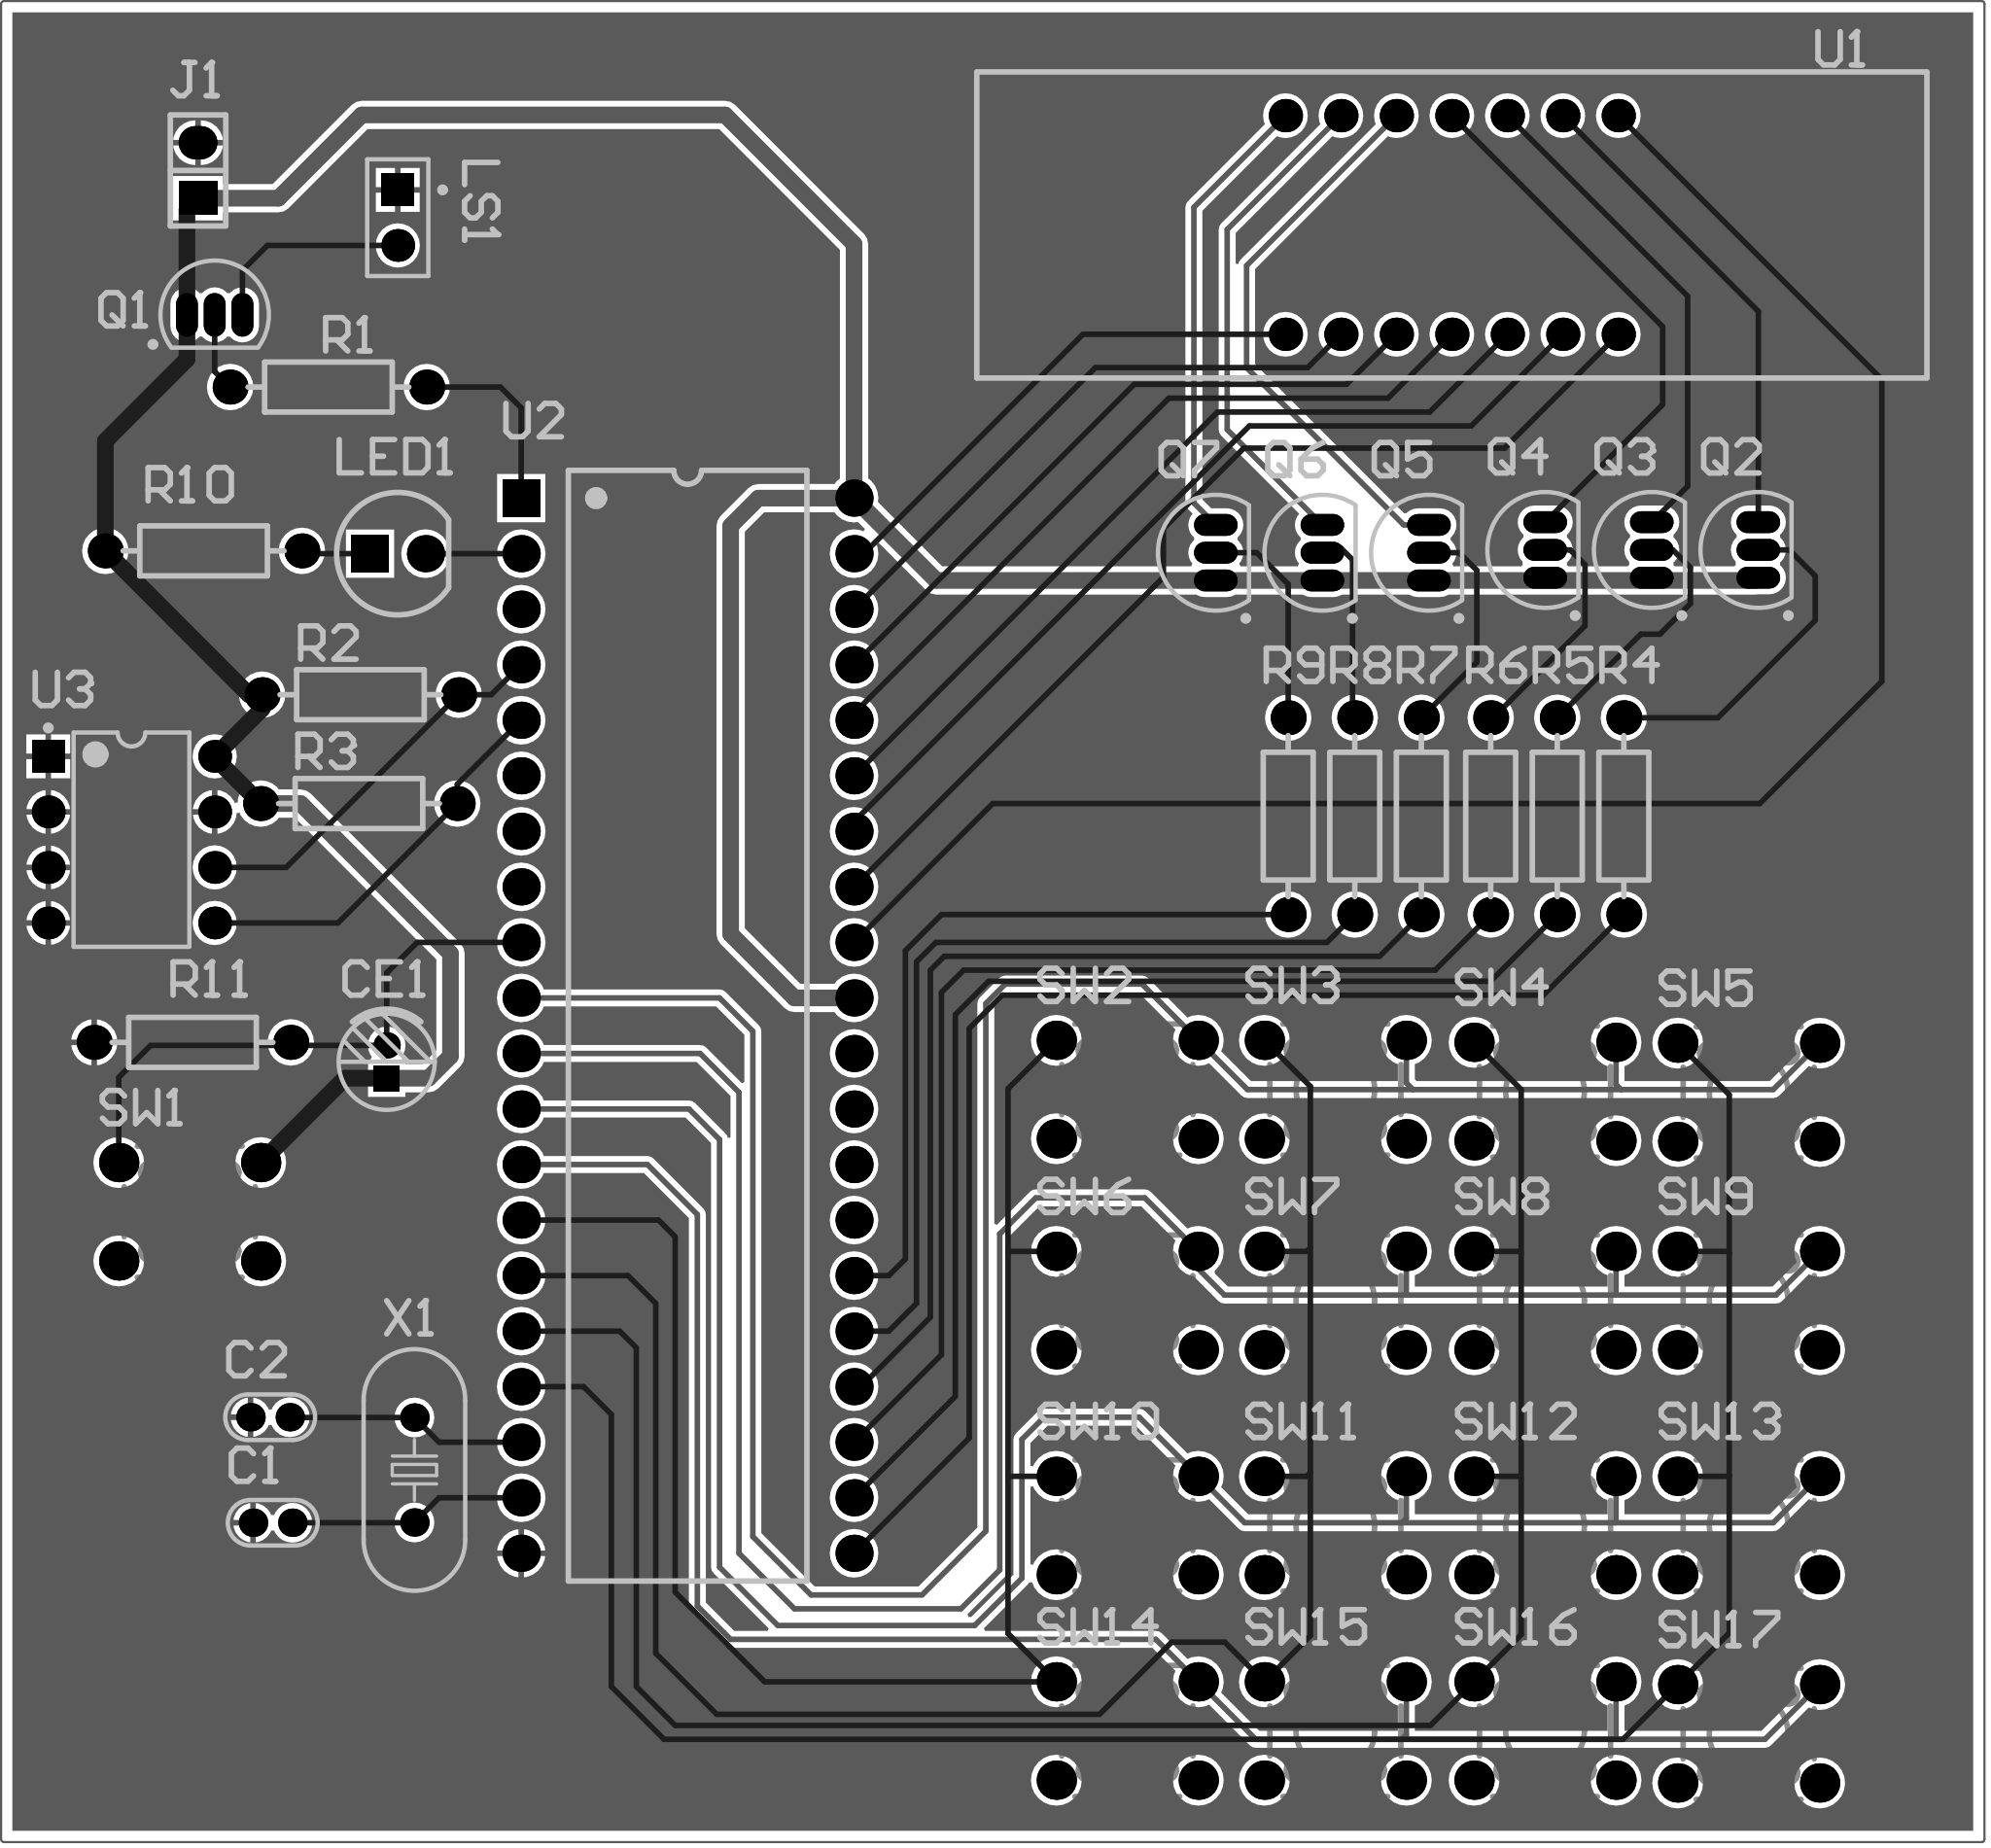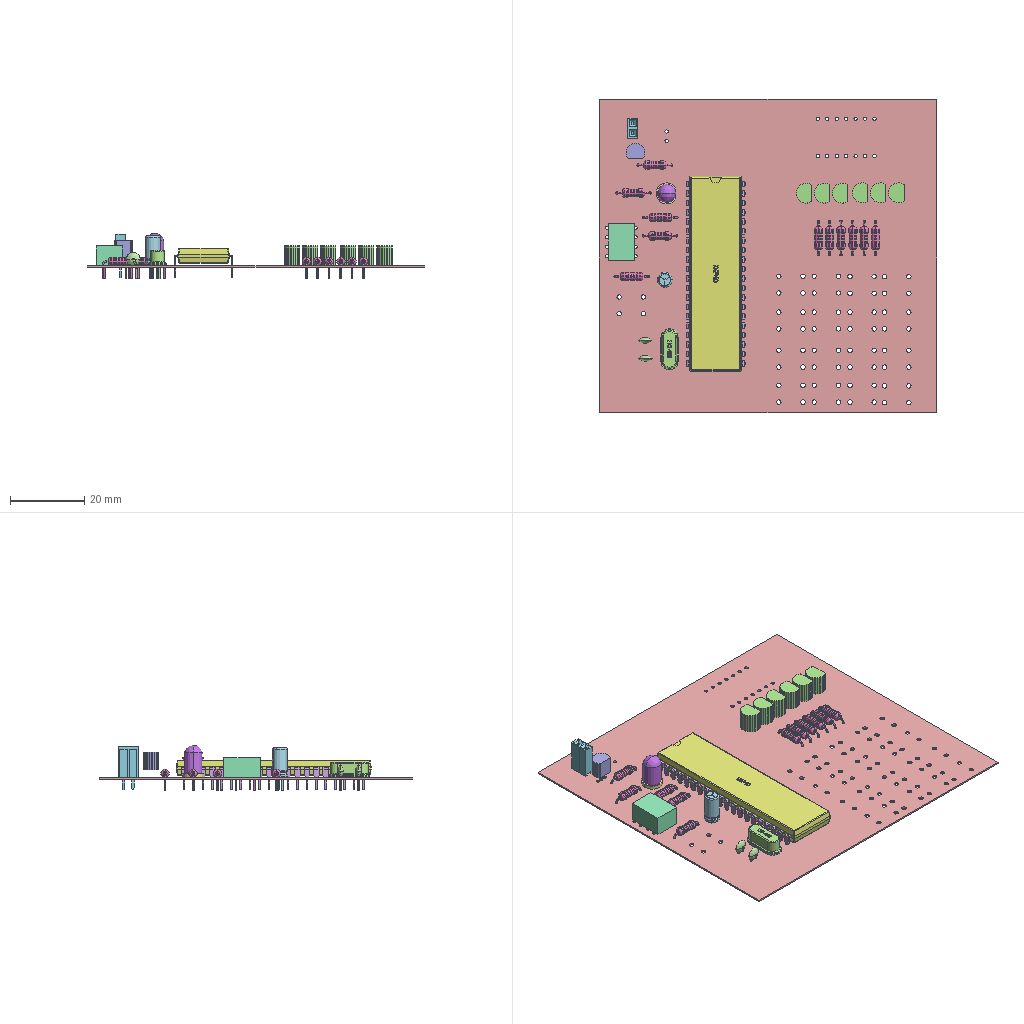Circuit board layout | Altium Designer | box 90.8 x 84.2 x 12.3 mm
Layer stack:
# Altium Designer layer stack of  (unit mm; dielectric type: 0 none, 1 core, 2 prepreg, 3 surface material)
index,name,kind,layer,copper_thickness_mm,dielectric_type,dielectric_thickness_mm,dielectric_material,dielectric_constant
0,Top Paste,other,,,,,,
1,Top Overlay,other,,,,,,
2,Top Solder,dielectric,,,3,0.0102,Solder Resist,3.5
3,Top Layer,copper,Top Layer,0.0356,,,,
4,Dielectric 1,dielectric,,,0,0.32,FR-4,4.8
5,Bottom Layer,copper,Bottom Layer,0.0356,,,,
6,Bottom Solder,dielectric,,,3,0.0102,Solder Resist,3.5
7,Bottom Overlay,other,,,,,,
8,Bottom Paste,other,,,,,,
# drill layer pairs: low layer,high layer
drill_pair,Top Layer,Bottom Layer
Part placement:
Designator,Comment,Layer,Footprint,Center-X(mm),Center-Y(mm),Rotation
C1,30PF,TopLayer,CC_1.8*3.6,35.422,57.531,0
C2,30PF,TopLayer,CC_1.8*3.6,35.306,62.357,0
CE1,47UF,TopLayer,CAP_1.5*4*8,40.64,78.613,90
LED1,Red,TopLayer,LED_5MM-B,41.148,101.854,0
LS1,Bell,TopLayer,PIN2,41.148,117.221,270
Q1,PNP,TopLayer,TO-92A,32.766,112.776,270
Q2,NPN,TopLayer,TO-226-AA,103.44,102.025,360
Q3,NPN,TopLayer,TO-226-AA,98.561,102.025,360
Q4,NPN,TopLayer,TO-226-AA,93.682,102.025,360
Q5,NPN,TopLayer,TO-226-AA,88.359,101.898,360
Q6,NPN,TopLayer,TO-226-AA,83.48,101.898,360
Q7,NPN,TopLayer,TO-226-AA,78.601,101.898,360
R1,470,TopLayer,RS_1/4W,37.973,109.474,180
R2,10K,TopLayer,RS_1/4W,39.438,95.403,180
R3,10K,TopLayer,RS_1/4W,39.37,90.424,180
R4,1K,TopLayer,RS_1/4W,97.282,89.848,90
R5,1K,TopLayer,RS_1/4W,94.234,89.848,90
R6,1K,TopLayer,RS_1/4W,91.186,89.848,90
R7,1K,TopLayer,RS_1/4W,88.011,89.848,90
R8,1K,TopLayer,RS_1/4W,84.963,89.848,90
R9,1K,TopLayer,RS_1/4W,81.915,89.848,90
R10,100,TopLayer,RS_1/4W,32.258,101.981,180
R11,1K,TopLayer,RS_1/4W,31.75,79.502,360
SW1,3x6x5,TopLayer,四脚轻触开关,31.623,71.755,0
SW2,3x6x5,TopLayer,四脚轻触开关,74.549,77.343,360
SW3,3x6x5,TopLayer,四脚轻触开关,84.074,77.343,360
SW4,3x6x5,TopLayer,四脚轻触开关,93.674,77.252,360
SW5,3x6x5,TopLayer,四脚轻触开关,102.997,77.216,360
SW6,3x6x5,TopLayer,四脚轻触开关,74.549,67.691,360
SW7,3x6x5,TopLayer,四脚轻触开关,84.074,67.691,360
SW8,3x6x5,TopLayer,四脚轻触开关,93.674,67.691,360
SW9,3x6x5,TopLayer,四脚轻触开关,102.997,67.691,360
SW10,3x6x5,TopLayer,四脚轻触开关,74.549,57.404,360
SW11,3x6x5,TopLayer,四脚轻触开关,84.074,57.404,360
SW12,3x6x5,TopLayer,四脚轻触开关,93.674,57.404,360
SW13,3x6x5,TopLayer,四脚轻触开关,102.997,57.404,360
SW14,3x6x5,TopLayer,四脚轻触开关,74.549,48.006,360
SW15,3x6x5,TopLayer,四脚轻触开关,84.074,48.006,360
SW16,3x6x5,TopLayer,四脚轻触开关,93.674,48.006,360
SW17,3x6x5,TopLayer,四脚轻触开关,102.997,47.879,360
U1,6-digit display_1,TopLayer,6位数码管,89.408,116.887,360
U2,ATC89C52,TopLayer,DIP40,54.419,80.264,0
U3,24C02C,TopLayer,PDIP300-P8,28.956,88.773,0
X1,12MHz,TopLayer,OSC_HC-49S,41.91,59.944,270
J1,Female HDR1X2,TopLayer,Fe-HDR1X2/2.54-S,32.004,119.38,90
Pad and via stacks:
# Altium Designer via and pad stacks of  (unit mm). Each distinct definition once, with the count of objects using it.
# via: kind,start_layer,end_layer,hole_mm,diameter_mm,mode(0 simple;1 top-mid-bottom;2 full stack),diameter_per_layer,count,example_net
# pad: kind,layer,hole_mm,hole_type(0 round;1 square;2 slot),plating,top_size,top_shape(1 round;2 rect;3 octagon;9 rounded rect),mid_size,bottom_size,mode,footprint,size_per_layer,count,example
pad,Multi-Layer,1.2,0,plated,1.8x1.8,1,1.8x1.8,1.8x1.8,0,\u00CB\u00C4\u00BD\u00C5\u00C7\u00E1\u00B4\u00A5\u00BF\u00AA\u00B9\u00D8,,68,SW14.1
pad,Multi-Layer,0.6,0,plated,1.6x1.6,1,1.6x1.6,1.6x1.6,0,RS 1/4W,,22,R11.1
pad,Multi-Layer,0.6,0,plated,1.2x1.2,2,1.2x1.2,1.2x1.2,0,CAP 1.5*4*8,,1,CE1.1
pad,Multi-Layer,0.6,0,plated,1.2x1.2,1,1.2x1.2,1.2x1.2,0,CAP 1.5*4*8,,1,CE1.2
pad,Multi-Layer,0.5,0,plated,1.3x1.3,1,1.3x1.3,1.3x1.3,0,CC 1.8*3.6,,4,C2.1
pad,Multi-Layer,0.6,0,plated,1.3x1.3,1,1.3x1.3,1.3x1.3,0,OSC HC-49S,,2,X1.1
pad,Multi-Layer,0.9,0,plated,1.7x1.7,1,1.7x1.7,1.7x1.7,0,LED 5MM-B,,1,LED1.2
pad,Multi-Layer,0.9,0,plated,1.7x1.7,2,1.7x1.7,1.7x1.7,0,LED 5MM-B,,1,LED1.1
pad,Multi-Layer,0.9,0,plated,1.5x1.5,2,1.5x1.5,1.5x1.5,0,PDIP300-P8,,1,U3.1
pad,Multi-Layer,0.9,0,plated,1.5x1.5,1,1.5x1.5,1.5x1.5,0,PDIP300-P8,,7,U3.2
pad,Multi-Layer,0.9,0,plated,2x1,1,2x1,2x1,0,TO-226-AA,,18,Q2.3
pad,Multi-Layer,0.8,0,plated,1.7x1.7,2,1.7x1.7,1.7x1.7,0,DIP40,,1,U2.1
pad,Multi-Layer,0.8,0,plated,1.7x1.7,1,1.7x1.7,1.7x1.7,0,DIP40,,39,U2.2
pad,Multi-Layer,0.9,0,plated,2x1,1,2x1,2x1,0,TO-92A,,3,Q1.1
pad,Multi-Layer,0.9,0,plated,1.5x1.5,1,1.5x1.5,1.5x1.5,0,PIN2,,1,LS1.2
pad,Multi-Layer,0.9,0,plated,1.5x1.5,2,1.5x1.5,1.5x1.5,0,PIN2,,1,LS1.1
pad,Multi-Layer,0.9144,0,plated,1.524x1.524,1,1.524x1.524,1.524x1.524,0,6\u00CE\u00BB\u00CA\u00FD\u00C2\u00EB\u00B9\u00DC,,14,U1.1
pad,Multi-Layer,0.8128,0,plated,1.524x1.778,1,1.524x1.778,1.524x1.778,0,Fe-HDR1X2/2.54-S,,1,J1.2
pad,Multi-Layer,0.8128,0,plated,1.524x1.778,2,1.524x1.778,1.524x1.778,0,Fe-HDR1X2/2.54-S,,1,J1.1
Copper pours:
name,layer,net,type(0 solid;1 hatched;2 none)
D,Bottom Layer,GND,0
Design rules, without the lines most boards share:
# Altium Designer design rules of  (exported by Altium Designer, unit mm)
# columns: name | kind | enabled | priority | scope1 | scope2 | descriptor | typed fields (field=value)
SilkToSilkClearance | 55 | enabled | 1 | All | All | Silk to Silk (Clearance=0mil) (All),(All) |
SilkToSolderMaskClearance | 54 | enabled | 1 | IsPad | All | Silk To Solder Mask (Clearance=0mil) (IsPad),(All) |
MinimumSolderMaskSliver | 53 | enabled | 1 | All | All | Minimum Solder Mask Sliver (Gap=0mil) (All),(All) |
HoleToHoleClearance | 52 | enabled | 1 | All | All | Hole To Hole Clearance (Gap=10mil) (All),(All) | gap=0.254
DiffPairsRouting | 51 | enabled | 1 | All | All | Differential Pairs Uncoupled Length using the Gap Constraints (Min=10mil) (Max=10mil) (Prefered=10mil)  and Width Constraints (Min=15mil) (Max=15mil) (Prefered=15mil) (All) |
SolderMaskExpansion | 13 | enabled | 1 | All | All | Solder Mask Expansion (Expansion =4mil) (All) | expansion=0.1016
PasteMaskExpansion | 14 | enabled | 1 | All | All | Paste Mask Expansion (Expansion =0mil) (All) | expansion=0
RoutingVias | 11 | enabled | 1 | All | All | Routing Via (MinHoleWidth=28mil) (MaxHoleWidth=28mil) (PreferredHoleWidth=28mil) (MinWidth=50mil) (MaxWidth=50mil) (PreferedWidth=50mil) (All) | via_min_hole=0.7112 via_max_hole=0.7112 via_preferred_diameter=1.27 via_preferred_hole=0.7112
Width | 2 | enabled | 1 | All | All | Width Constraint (Min=10mil) (Max=30mil) (Preferred=10mil) (All) |
PolygonConnect | 20 | enabled | 1 | All | All | Polygon Connect Rule(Relief Connect )(Conductor Width=10mil) (Relief Angle=90 Angle) (Entries=4) (Air Gap Width=10mil) (All),(All) | connect_style(0=relief,1=direct,2=none)=0 relief_conductor_width=0.254 relief_entries=4
PlaneConnect | 6 | enabled | 1 | All | All | Power Plane Connect Rule(Relief Connect )(Expansion=20mil) (Conductor Width=10mil) (Air Gap=10mil) (Entries=4) (All) | relief_conductor_width=0.254 relief_entries=4 relief_expansion=0.508
Clearance | 0 | enabled | 1 | All | All | Clearance Constraint (Gap=10mil) (All),(All) | gap=0.254